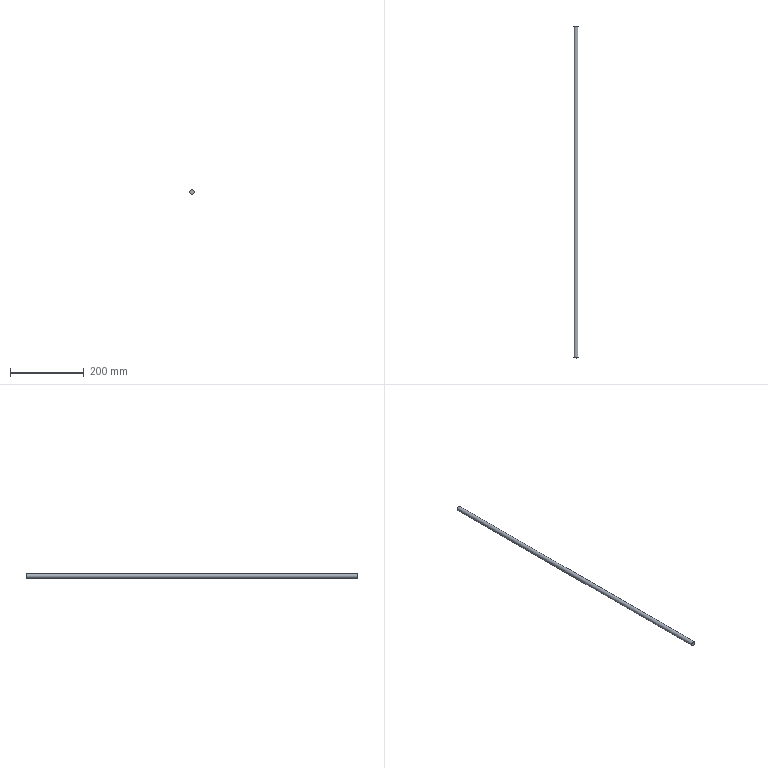Part | STEP file | solid 176 | 1 solid | 3 faces | box 12 x 900 x 12 mm | volume 101788 mm3 | plane 2 | cylinder 1 | commonest cylinder face diameters 12 x1